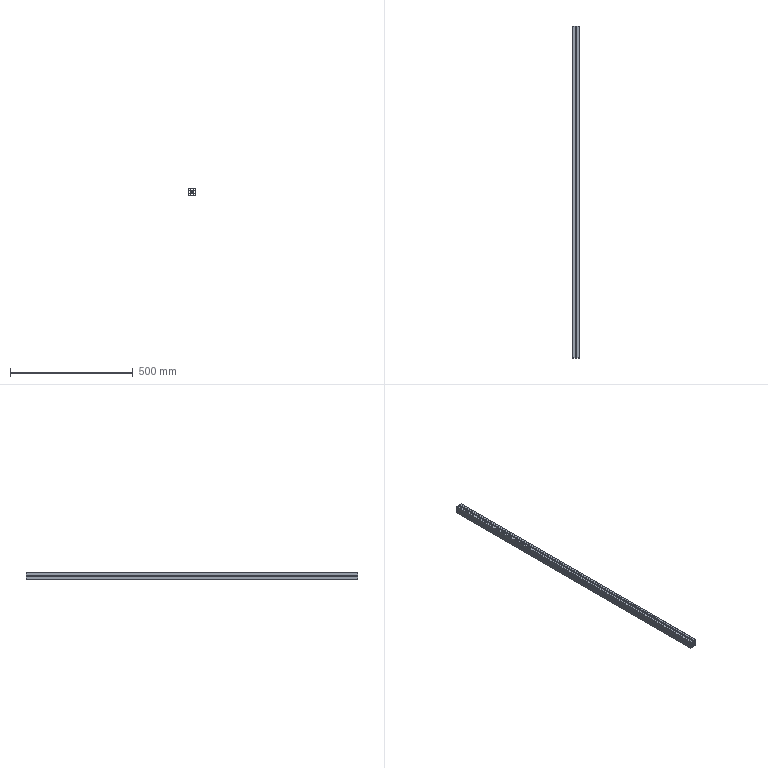Part | STEP file | 08-05 Guard bracket 5 | 1 solid | 68 faces | box 30 x 1350 x 30 mm | volume 570688 mm3 | plane 54 | cylinder 14 | commonest cylinder face diameters 6 x10 2 x4